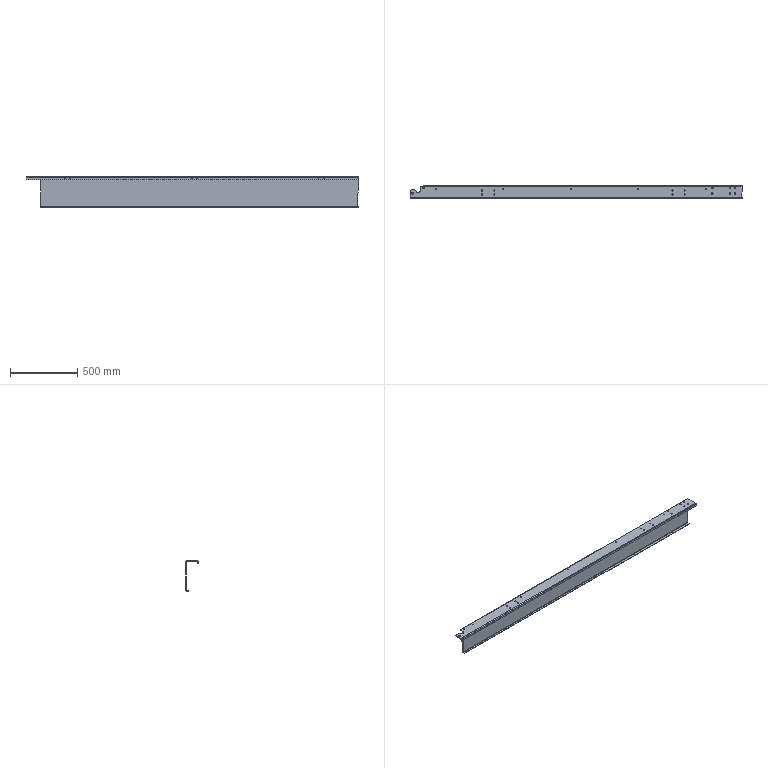Part | STEP file | Flat conveyor mechanism-CN2500x400-103-101a | 1 solid | 102 faces | box 2460 x 93 x 223 mm | volume 2426362 mm3 | cylinder 76 | plane 25 | spline 1 | commonest cylinder face diameters 6 x27 9 x16 11 x16 7 x10 12 x3 20 x2